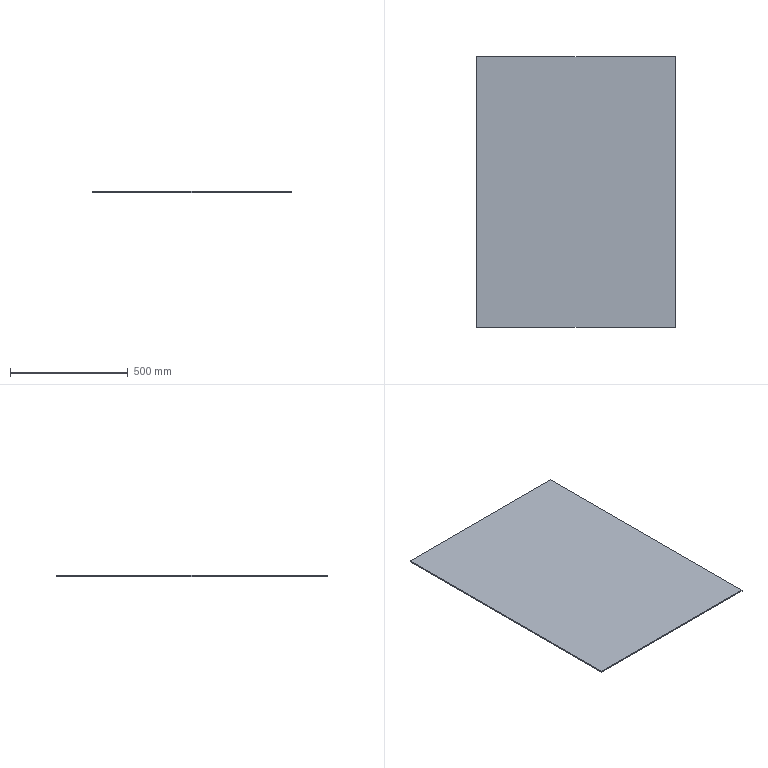Part | STEP file | 750038318 | 1 solid | 6 faces | box 845 x 1149 x 5 mm | volume 4854525 mm3 | plane 6
STEP:
#1=CARTESIAN_POINT('',(422.5,1149.,5.));
#2=VERTEX_POINT('',#1);
#3=CARTESIAN_POINT('',(422.5,0.,5.));
#4=VERTEX_POINT('',#3);
#5=CARTESIAN_POINT('',(422.5,0.,5.));
#6=DIRECTION('',(0.,-1.,0.));
#7=VECTOR('',#6,1000.);
#8=LINE('',#5,#7);
#9=EDGE_CURVE('',#2,#4,#8,.T.);
#10=ORIENTED_EDGE('',*,*,#9,.F.);
#11=CARTESIAN_POINT('',(-422.5,1149.,5.));
#12=VERTEX_POINT('',#11);
#13=CARTESIAN_POINT('',(0.,1149.,5.));
#14=DIRECTION('',(1.,0.,0.));
#15=VECTOR('',#14,1000.);
#16=LINE('',#13,#15);
#17=EDGE_CURVE('',#12,#2,#16,.T.);
#18=ORIENTED_EDGE('',*,*,#17,.F.);
#19=CARTESIAN_POINT('',(-422.5,0.,5.));
#20=VERTEX_POINT('',#19);
#21=CARTESIAN_POINT('',(-422.5,0.,5.));
#22=DIRECTION('',(0.,1.,0.));
#23=VECTOR('',#22,1000.);
#24=LINE('',#21,#23);
#25=EDGE_CURVE('',#20,#12,#24,.T.);
#26=ORIENTED_EDGE('',*,*,#25,.F.);
#27=CARTESIAN_POINT('',(0.,0.,5.));
#28=DIRECTION('',(-1.,0.,0.));
#29=VECTOR('',#28,1000.);
#30=LINE('',#27,#29);
#31=EDGE_CURVE('',#4,#20,#30,.T.);
#32=ORIENTED_EDGE('',*,*,#31,.F.);
#33=EDGE_LOOP('',(#10,#18,#26,#32));
#34=FACE_OUTER_BOUND('',#33,.T.);
#35=CARTESIAN_POINT('',(0.,0.,5.));
#36=DIRECTION('',(0.,0.,-1.));
#37=DIRECTION('',(-1.,0.,0.));
#38=AXIS2_PLACEMENT_3D('',#35,#36,#37);
#39=PLANE('',#38);
#40=ADVANCED_FACE('',(#34),#39,.F.);
#41=ORIENTED_EDGE('',*,*,#31,.T.);
#42=CARTESIAN_POINT('',(-422.5,0.,0.));
#43=VERTEX_POINT('',#42);
#44=CARTESIAN_POINT('',(-422.5,0.,5.));
#45=DIRECTION('',(0.,0.,-1.));
#46=VECTOR('',#45,1000.);
#47=LINE('',#44,#46);
#48=EDGE_CURVE('',#20,#43,#47,.T.);
#49=ORIENTED_EDGE('',*,*,#48,.T.);
#50=CARTESIAN_POINT('',(422.5,0.,0.));
#51=VERTEX_POINT('',#50);
#52=CARTESIAN_POINT('',(422.5,0.,0.));
#53=DIRECTION('',(1.,0.,0.));
#54=VECTOR('',#53,1000.);
#55=LINE('',#52,#54);
#56=EDGE_CURVE('',#43,#51,#55,.T.);
#57=ORIENTED_EDGE('',*,*,#56,.T.);
#58=CARTESIAN_POINT('',(422.5,0.,5.));
#59=DIRECTION('',(0.,0.,1.));
#60=VECTOR('',#59,1000.);
#61=LINE('',#58,#60);
#62=EDGE_CURVE('',#51,#4,#61,.T.);
#63=ORIENTED_EDGE('',*,*,#62,.T.);
#64=EDGE_LOOP('',(#41,#49,#57,#63));
#65=FACE_OUTER_BOUND('',#64,.T.);
#66=CARTESIAN_POINT('',(422.5,0.,5.));
#67=DIRECTION('',(0.,-1.,0.));
#68=DIRECTION('',(0.,0.,-1.));
#69=AXIS2_PLACEMENT_3D('',#66,#67,#68);
#70=PLANE('',#69);
#71=ADVANCED_FACE('',(#65),#70,.T.);
#72=ORIENTED_EDGE('',*,*,#9,.T.);
#73=ORIENTED_EDGE('',*,*,#62,.F.);
#74=CARTESIAN_POINT('',(422.5,1149.,0.));
#75=VERTEX_POINT('',#74);
#76=CARTESIAN_POINT('',(422.5,1149.,0.));
#77=DIRECTION('',(0.,1.,0.));
#78=VECTOR('',#77,1000.);
#79=LINE('',#76,#78);
#80=EDGE_CURVE('',#51,#75,#79,.T.);
#81=ORIENTED_EDGE('',*,*,#80,.T.);
#82=CARTESIAN_POINT('',(422.5,1149.,5.));
#83=DIRECTION('',(0.,0.,1.));
#84=VECTOR('',#83,1000.);
#85=LINE('',#82,#84);
#86=EDGE_CURVE('',#75,#2,#85,.T.);
#87=ORIENTED_EDGE('',*,*,#86,.T.);
#88=EDGE_LOOP('',(#72,#73,#81,#87));
#89=FACE_OUTER_BOUND('',#88,.T.);
#90=CARTESIAN_POINT('',(422.5,1149.,5.));
#91=DIRECTION('',(1.,0.,0.));
#92=DIRECTION('',(0.,0.,-1.));
#93=AXIS2_PLACEMENT_3D('',#90,#91,#92);
#94=PLANE('',#93);
#95=ADVANCED_FACE('',(#89),#94,.T.);
#96=ORIENTED_EDGE('',*,*,#17,.T.);
#97=ORIENTED_EDGE('',*,*,#86,.F.);
#98=CARTESIAN_POINT('',(-422.5,1149.,0.));
#99=VERTEX_POINT('',#98);
#100=CARTESIAN_POINT('',(-422.5,1149.,0.));
#101=DIRECTION('',(-1.,0.,0.));
#102=VECTOR('',#101,1000.);
#103=LINE('',#100,#102);
#104=EDGE_CURVE('',#75,#99,#103,.T.);
#105=ORIENTED_EDGE('',*,*,#104,.T.);
#106=CARTESIAN_POINT('',(-422.5,1149.,5.));
#107=DIRECTION('',(0.,0.,1.));
#108=VECTOR('',#107,1000.);
#109=LINE('',#106,#108);
#110=EDGE_CURVE('',#99,#12,#109,.T.);
#111=ORIENTED_EDGE('',*,*,#110,.T.);
#112=EDGE_LOOP('',(#96,#97,#105,#111));
#113=FACE_OUTER_BOUND('',#112,.T.);
#114=CARTESIAN_POINT('',(-422.5,1149.,5.));
#115=DIRECTION('',(0.,1.,0.));
#116=DIRECTION('',(0.,0.,1.));
#117=AXIS2_PLACEMENT_3D('',#114,#115,#116);
#118=PLANE('',#117);
#119=ADVANCED_FACE('',(#113),#118,.T.);
#120=ORIENTED_EDGE('',*,*,#25,.T.);
#121=ORIENTED_EDGE('',*,*,#110,.F.);
#122=CARTESIAN_POINT('',(-422.5,0.,0.));
#123=DIRECTION('',(0.,-1.,0.));
#124=VECTOR('',#123,1000.);
#125=LINE('',#122,#124);
#126=EDGE_CURVE('',#99,#43,#125,.T.);
#127=ORIENTED_EDGE('',*,*,#126,.T.);
#128=ORIENTED_EDGE('',*,*,#48,.F.);
#129=EDGE_LOOP('',(#120,#121,#127,#128));
#130=FACE_OUTER_BOUND('',#129,.T.);
#131=CARTESIAN_POINT('',(-422.5,0.,5.));
#132=DIRECTION('',(-1.,0.,0.));
#133=DIRECTION('',(0.,0.,1.));
#134=AXIS2_PLACEMENT_3D('',#131,#132,#133);
#135=PLANE('',#134);
#136=ADVANCED_FACE('',(#130),#135,.T.);
#137=ORIENTED_EDGE('',*,*,#104,.F.);
#138=ORIENTED_EDGE('',*,*,#80,.F.);
#139=ORIENTED_EDGE('',*,*,#56,.F.);
#140=ORIENTED_EDGE('',*,*,#126,.F.);
#141=EDGE_LOOP('',(#137,#138,#139,#140));
#142=FACE_OUTER_BOUND('',#141,.T.);
#143=CARTESIAN_POINT('',(0.,0.,0.));
#144=DIRECTION('',(0.,0.,-1.));
#145=DIRECTION('',(-1.,0.,0.));
#146=AXIS2_PLACEMENT_3D('',#143,#144,#145);
#147=PLANE('',#146);
#148=ADVANCED_FACE('',(#142),#147,.T.);
#149=CLOSED_SHELL('',(#40,#71,#95,#119,#136,#148));
#150=MANIFOLD_SOLID_BREP('',#149);
#151=CARTESIAN_POINT('',(0.,0.,0.));
#152=DIRECTION('',(0.,0.,1.));
#153=DIRECTION('',(1.,0.,0.));
#154=AXIS2_PLACEMENT_3D('',#151,#152,#153);
#155=(LENGTH_UNIT()NAMED_UNIT(*)SI_UNIT(.MILLI.,.METRE.));
#156=UNCERTAINTY_MEASURE_WITH_UNIT(LENGTH_MEASURE(0.00001),#155,'','');
#157=(NAMED_UNIT(*)PLANE_ANGLE_UNIT()SI_UNIT($,.RADIAN.));
#158=(NAMED_UNIT(*)SI_UNIT($,.STERADIAN.)SOLID_ANGLE_UNIT());
#159=(GEOMETRIC_REPRESENTATION_CONTEXT(3)GLOBAL_UNCERTAINTY_ASSIGNED_CONTEXT((#156))GLOBAL_UNIT_ASSIGNED_CONTEXT((#155,#157,#158))REPRESENTATION_CONTEXT('',''));
#160=ADVANCED_BREP_SHAPE_REPRESENTATION('',(#150,#154),#159);